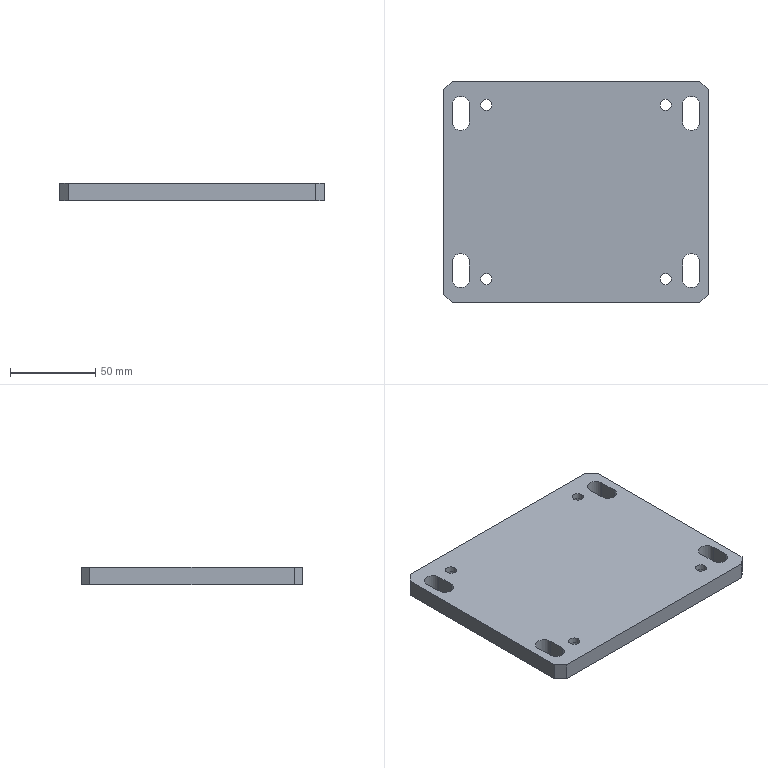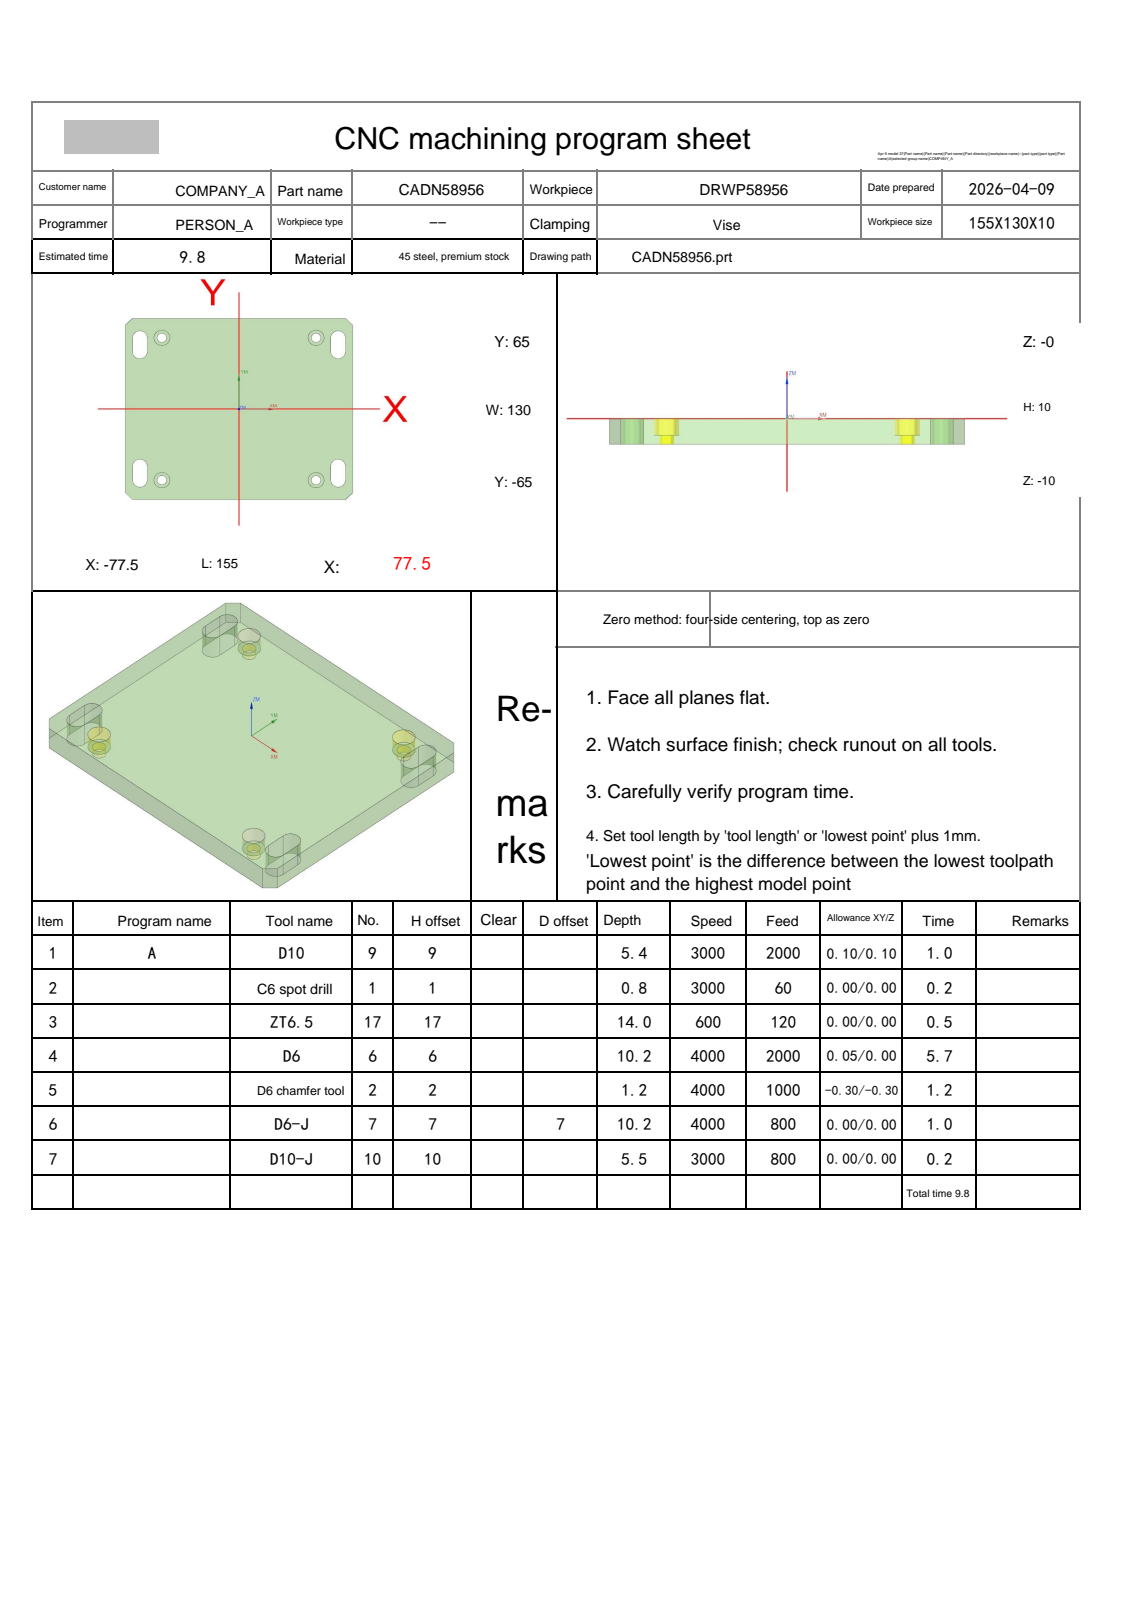NC program | NX | posted by the shop | part box 155 x 130 x 10 mm
Lines 1 to 1868 of 2515, first 1318 of 1866 lines:
%
O0001
(Machine time: 11.12 MIN)
(===Total Tool:7===)
(T9=D10     D=10.  R=0.   D-  H09 Z=-5.4  )
(T1=C6 spot drill   D=6.   R=0.   D-  H01 Z=-0.8  )
(T17=ZT6.5  D=6.5  DR_a=118 D-  H17 Z=-13.95)
(T6=D6      D=6.   R=0.   D-  H06 Z=-10.2 )
(T2=D6 chamfer tool   D=6.   R=0.   D-  H02 Z=-1.2  )
(T7=D6-J    D=6.   R=0.   D7  H07 Z=-10.2 )
(T10=D10-J  D=10.  R=0.   D-  H10 Z=-5.5  )
G80 G90 G17 G49 G40
G91 G28 Z0
M01
N1 T09 M06
(D10  D=10. R=0. H=09 ce=0.10 di=0.10)
G00 G90 G54 X-69.742 Y-74.97 M03 S3000
G43 H09 Z20.
M08
Z-.3
G01 X-76.106 Y-68.606 F2000.
X-81.106 Y-63.606
X-87.47 Y-57.242
G00 Z-.6
G01 X-81.106 Y-63.606
X-76.106 Y-68.606
X-69.742 Y-74.97
G00 Z-.9
G01 X-76.106 Y-68.606
X-81.106 Y-63.606
X-87.47 Y-57.242
G00 Z-1.2
G01 X-81.106 Y-63.606
X-76.106 Y-68.606
X-69.742 Y-74.97
G00 Z-1.5
G01 X-76.106 Y-68.606
X-81.106 Y-63.606
X-87.47 Y-57.242
G00 Z-1.8
G01 X-81.106 Y-63.606
X-76.106 Y-68.606
X-69.742 Y-74.97
G00 Z-2.1
G01 X-76.106 Y-68.606
X-81.106 Y-63.606
X-87.47 Y-57.242
G00 Z-2.4
G01 X-81.106 Y-63.606
X-76.106 Y-68.606
X-69.742 Y-74.97
G00 Z-2.7
G01 X-76.106 Y-68.606
X-81.106 Y-63.606
X-87.47 Y-57.242
G00 Z-3.
G01 X-81.106 Y-63.606
X-76.106 Y-68.606
X-69.742 Y-74.97
G00 Z-3.3
G01 X-76.106 Y-68.606
X-81.106 Y-63.606
X-87.47 Y-57.242
G00 Z-3.6
G01 X-81.106 Y-63.606
X-76.106 Y-68.606
X-69.742 Y-74.97
G00 Z-3.9
G01 X-76.106 Y-68.606
X-81.106 Y-63.606
X-87.47 Y-57.242
G00 Z-4.2
G01 X-81.106 Y-63.606
X-76.106 Y-68.606
X-69.742 Y-74.97
G00 Z-4.5
G01 X-76.106 Y-68.606
X-81.106 Y-63.606
X-87.47 Y-57.242
G00 Z-4.8
G01 X-81.106 Y-63.606
X-76.106 Y-68.606
X-69.742 Y-74.97
G00 Z-5.1
G01 X-76.106 Y-68.606
X-81.106 Y-63.606
X-87.47 Y-57.242
G00 Z-5.4
G01 X-81.106 Y-63.606
X-76.106 Y-68.606
X-69.742 Y-74.97
G00 Z20.
X-87.47 Y57.242
Z-.3
G01 X-81.106 Y63.606
X-76.106 Y68.606
X-69.742 Y74.97
G00 Z-.6
G01 X-76.106 Y68.606
X-81.106 Y63.606
X-87.47 Y57.242
G00 Z-.9
G01 X-81.106 Y63.606
X-76.106 Y68.606
X-69.742 Y74.97
G00 Z-1.2
G01 X-76.106 Y68.606
X-81.106 Y63.606
X-87.47 Y57.242
G00 Z-1.5
G01 X-81.106 Y63.606
X-76.106 Y68.606
X-69.742 Y74.97
G00 Z-1.8
G01 X-76.106 Y68.606
X-81.106 Y63.606
X-87.47 Y57.242
G00 Z-2.1
G01 X-81.106 Y63.606
X-76.106 Y68.606
X-69.742 Y74.97
G00 Z-2.4
G01 X-76.106 Y68.606
X-81.106 Y63.606
X-87.47 Y57.242
G00 Z-2.7
G01 X-81.106 Y63.606
X-76.106 Y68.606
X-69.742 Y74.97
G00 Z-3.
G01 X-76.106 Y68.606
X-81.106 Y63.606
X-87.47 Y57.242
G00 Z-3.3
G01 X-81.106 Y63.606
X-76.106 Y68.606
X-69.742 Y74.97
G00 Z-3.6
G01 X-76.106 Y68.606
X-81.106 Y63.606
X-87.47 Y57.242
G00 Z-3.9
G01 X-81.106 Y63.606
X-76.106 Y68.606
X-69.742 Y74.97
G00 Z-4.2
G01 X-76.106 Y68.606
X-81.106 Y63.606
X-87.47 Y57.242
G00 Z-4.5
G01 X-81.106 Y63.606
X-76.106 Y68.606
X-69.742 Y74.97
G00 Z-4.8
G01 X-76.106 Y68.606
X-81.106 Y63.606
X-87.47 Y57.242
G00 Z-5.1
G01 X-81.106 Y63.606
X-76.106 Y68.606
X-69.742 Y74.97
G00 Z-5.4
G01 X-76.106 Y68.606
X-81.106 Y63.606
X-87.47 Y57.242
G00 Z20.
X69.742 Y74.97
Z-.3
G01 X76.106 Y68.606
X81.106 Y63.606
X87.47 Y57.242
G00 Z-.6
G01 X81.106 Y63.606
X76.106 Y68.606
X69.742 Y74.97
G00 Z-.9
G01 X76.106 Y68.606
X81.106 Y63.606
X87.47 Y57.242
G00 Z-1.2
G01 X81.106 Y63.606
X76.106 Y68.606
X69.742 Y74.97
G00 Z-1.5
G01 X76.106 Y68.606
X81.106 Y63.606
X87.47 Y57.242
G00 Z-1.8
G01 X81.106 Y63.606
X76.106 Y68.606
X69.742 Y74.97
G00 Z-2.1
G01 X76.106 Y68.606
X81.106 Y63.606
X87.47 Y57.242
G00 Z-2.4
G01 X81.106 Y63.606
X76.106 Y68.606
X69.742 Y74.97
G00 Z-2.7
G01 X76.106 Y68.606
X81.106 Y63.606
X87.47 Y57.242
G00 Z-3.
G01 X81.106 Y63.606
X76.106 Y68.606
X69.742 Y74.97
G00 Z-3.3
G01 X76.106 Y68.606
X81.106 Y63.606
X87.47 Y57.242
G00 Z-3.6
G01 X81.106 Y63.606
X76.106 Y68.606
X69.742 Y74.97
G00 Z-3.9
G01 X76.106 Y68.606
X81.106 Y63.606
X87.47 Y57.242
G00 Z-4.2
G01 X81.106 Y63.606
X76.106 Y68.606
X69.742 Y74.97
G00 Z-4.5
G01 X76.106 Y68.606
X81.106 Y63.606
X87.47 Y57.242
G00 Z-4.8
G01 X81.106 Y63.606
X76.106 Y68.606
X69.742 Y74.97
G00 Z-5.1
G01 X76.106 Y68.606
X81.106 Y63.606
X87.47 Y57.242
G00 Z-5.4
G01 X81.106 Y63.606
X76.106 Y68.606
X69.742 Y74.97
G00 Z20.
X87.47 Y-57.242
Z-.3
G01 X81.106 Y-63.606
X76.106 Y-68.606
X69.742 Y-74.97
G00 Z-.6
G01 X76.106 Y-68.606
X81.106 Y-63.606
X87.47 Y-57.242
G00 Z-.9
G01 X81.106 Y-63.606
X76.106 Y-68.606
X69.742 Y-74.97
G00 Z-1.2
G01 X76.106 Y-68.606
X81.106 Y-63.606
X87.47 Y-57.242
G00 Z-1.5
G01 X81.106 Y-63.606
X76.106 Y-68.606
X69.742 Y-74.97
G00 Z-1.8
G01 X76.106 Y-68.606
X81.106 Y-63.606
X87.47 Y-57.242
G00 Z-2.1
G01 X81.106 Y-63.606
X76.106 Y-68.606
X69.742 Y-74.97
G00 Z-2.4
G01 X76.106 Y-68.606
X81.106 Y-63.606
X87.47 Y-57.242
G00 Z-2.7
G01 X81.106 Y-63.606
X76.106 Y-68.606
X69.742 Y-74.97
G00 Z-3.
G01 X76.106 Y-68.606
X81.106 Y-63.606
X87.47 Y-57.242
G00 Z-3.3
G01 X81.106 Y-63.606
X76.106 Y-68.606
X69.742 Y-74.97
G00 Z-3.6
G01 X76.106 Y-68.606
X81.106 Y-63.606
X87.47 Y-57.242
G00 Z-3.9
G01 X81.106 Y-63.606
X76.106 Y-68.606
X69.742 Y-74.97
G00 Z-4.2
G01 X76.106 Y-68.606
X81.106 Y-63.606
X87.47 Y-57.242
G00 Z-4.5
G01 X81.106 Y-63.606
X76.106 Y-68.606
X69.742 Y-74.97
G00 Z-4.8
G01 X76.106 Y-68.606
X81.106 Y-63.606
X87.47 Y-57.242
G00 Z-5.1
G01 X81.106 Y-63.606
X76.106 Y-68.606
X69.742 Y-74.97
G00 Z-5.4
G01 X76.106 Y-68.606
X81.106 Y-63.606
X87.47 Y-57.242
G00 Z20.
G91 G28 Z0.0
M05
M09
G91 G28 Z0.0
M01
N2 T01 M06
(C6 spot drill D=6. R=0. H=01 ce=0.00 di=0.10)
G00 G90 G54 X-52.5 Y-51. M03 S3000
G43 H01 Z20.
M08
G98 G81 X-52.5 Y-51. Z-.8 R1. F60.
Y51.
X52.5
Y-51.
G80
G00 Z20.
G91 G28 Z0.0
M05
M09
G91 G28 Z0.0
M01
N3 T17 M06
(ZT6.5 D=6.5 DR_a=118 H=17)
G00 G90 G54 X-52.5 Y-51. M03 S600
G43 H17 Z20.
M08
G98 G83 X-52.5 Y-51. Z-13.953 R1. F120. Q2.
Y51.
X52.5
Y-51.
G80
G00 Z20.
G91 G28 Z0.0
M05
M09
G91 G28 Z0.0
M01
N4 T06 M06
(D6  D=6. R=0. H=06 ce=0.05 di=0.10)
G00 G90 G54 X-67.311 Y-52.95 M03 S4000
G43 H06 Z20.
M08
Z1.
G01 X-67.157 Z.992 F1500.
X-66.412 Y-52.654 Z.95
X-65.846 Y-52.088 Z.908
X-65.55 Y-51.343 Z.866
Y-40.657 Z.306
X-65.846 Y-39.912 Z.264
X-66.412 Y-39.346 Z.222
X-67.157 Y-39.05 Z.18
X-67.843 Z.144
X-68.588 Y-39.346 Z.102
X-69.154 Y-39.912 Z.06
X-69.45 Y-40.657 Z.018
Y-41. Z0.0
Y-51. Z-.062
G03 X-67.5 Y-52.95 Z-.081 I1.95 J0.0
X-65.55 Y-51. Z-.1 I0.0 J1.95
G01 Y-41. Z-.162
G03 X-67.5 Y-39.05 Z-.181 I-1.95 J0.0
X-69.45 Y-41. Z-.2 I0.0 J-1.95
G01 Y-51. Z-.262
G03 X-67.5 Y-52.95 Z-.281 I1.95 J0.0
X-65.55 Y-51. Z-.3 I0.0 J1.95
G01 Y-41. Z-.362
G03 X-67.5 Y-39.05 Z-.381 I-1.95 J0.0
X-69.45 Y-41. Z-.4 I0.0 J-1.95
G01 Y-51. Z-.462
G03 X-67.5 Y-52.95 Z-.481 I1.95 J0.0
X-65.55 Y-51. Z-.5 I0.0 J1.95
G01 Y-41. Z-.562
G03 X-67.5 Y-39.05 Z-.581 I-1.95 J0.0
X-69.45 Y-41. Z-.6 I0.0 J-1.95
G01 Y-51. Z-.662
G03 X-67.5 Y-52.95 Z-.681 I1.95 J0.0
X-65.55 Y-51. Z-.7 I0.0 J1.95
G01 Y-41. Z-.762
G03 X-67.5 Y-39.05 Z-.781 I-1.95 J0.0
X-69.45 Y-41. Z-.8 I0.0 J-1.95
G01 Y-51. Z-.862
G03 X-67.5 Y-52.95 Z-.881 I1.95 J0.0
X-65.55 Y-51. Z-.9 I0.0 J1.95
G01 Y-41. Z-.962
G03 X-67.5 Y-39.05 Z-.981 I-1.95 J0.0
X-69.45 Y-41. Z-1. I0.0 J-1.95
G01 Y-51. Z-1.062
G03 X-67.5 Y-52.95 Z-1.081 I1.95 J0.0
X-65.55 Y-51. Z-1.1 I0.0 J1.95
G01 Y-41. Z-1.162
G03 X-67.5 Y-39.05 Z-1.181 I-1.95 J0.0
X-69.45 Y-41. Z-1.2 I0.0 J-1.95
G01 Y-51. Z-1.262
G03 X-67.5 Y-52.95 Z-1.281 I1.95 J0.0
X-65.55 Y-51. Z-1.3 I0.0 J1.95
G01 Y-41. Z-1.362
G03 X-67.5 Y-39.05 Z-1.381 I-1.95 J0.0
X-69.45 Y-41. Z-1.4 I0.0 J-1.95
G01 Y-51. Z-1.462
G03 X-67.5 Y-52.95 Z-1.481 I1.95 J0.0
X-65.55 Y-51. Z-1.5 I0.0 J1.95
G01 Y-41. Z-1.562
G03 X-67.5 Y-39.05 Z-1.581 I-1.95 J0.0
X-69.45 Y-41. Z-1.6 I0.0 J-1.95
G01 Y-51. Z-1.662
G03 X-67.5 Y-52.95 Z-1.681 I1.95 J0.0
X-65.55 Y-51. Z-1.7 I0.0 J1.95
G01 Y-41. Z-1.762
G03 X-67.5 Y-39.05 Z-1.781 I-1.95 J0.0
X-69.45 Y-41. Z-1.8 I0.0 J-1.95
G01 Y-51. Z-1.862
G03 X-67.5 Y-52.95 Z-1.881 I1.95 J0.0
X-65.55 Y-51. Z-1.9 I0.0 J1.95
G01 Y-41. Z-1.962
G03 X-67.5 Y-39.05 Z-1.981 I-1.95 J0.0
X-69.45 Y-41. Z-2. I0.0 J-1.95
G01 Y-51. Z-2.062
G03 X-67.5 Y-52.95 Z-2.081 I1.95 J0.0
X-65.55 Y-51. Z-2.1 I0.0 J1.95
G01 Y-41. Z-2.162
G03 X-67.5 Y-39.05 Z-2.181 I-1.95 J0.0
X-69.45 Y-41. Z-2.2 I0.0 J-1.95
G01 Y-51. Z-2.262
G03 X-67.5 Y-52.95 Z-2.281 I1.95 J0.0
X-65.55 Y-51. Z-2.3 I0.0 J1.95
G01 Y-41. Z-2.362
G03 X-67.5 Y-39.05 Z-2.381 I-1.95 J0.0
X-69.45 Y-41. Z-2.4 I0.0 J-1.95
G01 Y-51. Z-2.462
G03 X-67.5 Y-52.95 Z-2.481 I1.95 J0.0
X-65.55 Y-51. Z-2.5 I0.0 J1.95
G01 Y-41. Z-2.562
G03 X-67.5 Y-39.05 Z-2.581 I-1.95 J0.0
X-69.45 Y-41. Z-2.6 I0.0 J-1.95
G01 Y-51. Z-2.662
G03 X-67.5 Y-52.95 Z-2.681 I1.95 J0.0
X-65.55 Y-51. Z-2.7 I0.0 J1.95
G01 Y-41. Z-2.762
G03 X-67.5 Y-39.05 Z-2.781 I-1.95 J0.0
X-69.45 Y-41. Z-2.8 I0.0 J-1.95
G01 Y-51. Z-2.862
G03 X-67.5 Y-52.95 Z-2.881 I1.95 J0.0
X-65.55 Y-51. Z-2.9 I0.0 J1.95
G01 Y-41. Z-2.962
G03 X-67.5 Y-39.05 Z-2.981 I-1.95 J0.0
X-69.45 Y-41. Z-3. I0.0 J-1.95
G01 Y-51. Z-3.062
G03 X-67.5 Y-52.95 Z-3.081 I1.95 J0.0
X-65.55 Y-51. Z-3.1 I0.0 J1.95
G01 Y-41. Z-3.162
G03 X-67.5 Y-39.05 Z-3.181 I-1.95 J0.0
X-69.45 Y-41. Z-3.2 I0.0 J-1.95
G01 Y-51. Z-3.262
G03 X-67.5 Y-52.95 Z-3.281 I1.95 J0.0
X-65.55 Y-51. Z-3.3 I0.0 J1.95
G01 Y-41. Z-3.362
G03 X-67.5 Y-39.05 Z-3.381 I-1.95 J0.0
X-69.45 Y-41. Z-3.4 I0.0 J-1.95
G01 Y-51. Z-3.462
G03 X-67.5 Y-52.95 Z-3.481 I1.95 J0.0
X-65.55 Y-51. Z-3.5 I0.0 J1.95
G01 Y-41. Z-3.562
G03 X-67.5 Y-39.05 Z-3.581 I-1.95 J0.0
X-69.45 Y-41. Z-3.6 I0.0 J-1.95
G01 Y-51. Z-3.662
G03 X-67.5 Y-52.95 Z-3.681 I1.95 J0.0
X-65.55 Y-51. Z-3.7 I0.0 J1.95
G01 Y-41. Z-3.762
G03 X-67.5 Y-39.05 Z-3.781 I-1.95 J0.0
X-69.45 Y-41. Z-3.8 I0.0 J-1.95
G01 Y-51. Z-3.862
G03 X-67.5 Y-52.95 Z-3.881 I1.95 J0.0
X-65.55 Y-51. Z-3.9 I0.0 J1.95
G01 Y-41. Z-3.962
G03 X-67.5 Y-39.05 Z-3.981 I-1.95 J0.0
X-69.45 Y-41. Z-4. I0.0 J-1.95
G01 Y-51. Z-4.062
G03 X-67.5 Y-52.95 Z-4.081 I1.95 J0.0
X-65.55 Y-51. Z-4.1 I0.0 J1.95
G01 Y-41. Z-4.162
G03 X-67.5 Y-39.05 Z-4.181 I-1.95 J0.0
X-69.45 Y-41. Z-4.2 I0.0 J-1.95
G01 Y-51. Z-4.262
G03 X-67.5 Y-52.95 Z-4.281 I1.95 J0.0
X-65.55 Y-51. Z-4.3 I0.0 J1.95
G01 Y-41. Z-4.362
G03 X-67.5 Y-39.05 Z-4.381 I-1.95 J0.0
X-69.45 Y-41. Z-4.4 I0.0 J-1.95
G01 Y-51. Z-4.462
G03 X-67.5 Y-52.95 Z-4.481 I1.95 J0.0
X-65.55 Y-51. Z-4.5 I0.0 J1.95
G01 Y-41. Z-4.562
G03 X-67.5 Y-39.05 Z-4.581 I-1.95 J0.0
X-69.45 Y-41. Z-4.6 I0.0 J-1.95
G01 Y-51. Z-4.662
G03 X-67.5 Y-52.95 Z-4.681 I1.95 J0.0
X-65.55 Y-51. Z-4.7 I0.0 J1.95
G01 Y-41. Z-4.762
G03 X-67.5 Y-39.05 Z-4.781 I-1.95 J0.0
X-69.45 Y-41. Z-4.8 I0.0 J-1.95
G01 Y-51. Z-4.862
G03 X-67.5 Y-52.95 Z-4.881 I1.95 J0.0
X-65.55 Y-51. Z-4.9 I0.0 J1.95
G01 Y-41. Z-4.962
G03 X-67.5 Y-39.05 Z-4.981 I-1.95 J0.0
X-69.45 Y-41. Z-5. I0.0 J-1.95
G01 Y-51. Z-5.062
G03 X-67.5 Y-52.95 Z-5.081 I1.95 J0.0
X-65.55 Y-51. Z-5.1 I0.0 J1.95
G01 Y-41. Z-5.162
G03 X-67.5 Y-39.05 Z-5.181 I-1.95 J0.0
X-69.45 Y-41. Z-5.2 I0.0 J-1.95
G01 Y-51. Z-5.262
G03 X-67.5 Y-52.95 Z-5.281 I1.95 J0.0
X-65.55 Y-51. Z-5.3 I0.0 J1.95
G01 Y-41. Z-5.362
G03 X-67.5 Y-39.05 Z-5.381 I-1.95 J0.0
X-69.45 Y-41. Z-5.4 I0.0 J-1.95
G01 Y-51. Z-5.462
G03 X-67.5 Y-52.95 Z-5.481 I1.95 J0.0
X-65.55 Y-51. Z-5.5 I0.0 J1.95
G01 Y-41. Z-5.562
G03 X-67.5 Y-39.05 Z-5.581 I-1.95 J0.0
X-69.45 Y-41. Z-5.6 I0.0 J-1.95
G01 Y-51. Z-5.662
G03 X-67.5 Y-52.95 Z-5.681 I1.95 J0.0
X-65.55 Y-51. Z-5.7 I0.0 J1.95
G01 Y-41. Z-5.762
G03 X-67.5 Y-39.05 Z-5.781 I-1.95 J0.0
X-69.45 Y-41. Z-5.8 I0.0 J-1.95
G01 Y-51. Z-5.862
G03 X-67.5 Y-52.95 Z-5.881 I1.95 J0.0
X-65.55 Y-51. Z-5.9 I0.0 J1.95
G01 Y-41. Z-5.962
G03 X-67.5 Y-39.05 Z-5.981 I-1.95 J0.0
X-69.45 Y-41. Z-6. I0.0 J-1.95
G01 Y-51. Z-6.062
G03 X-67.5 Y-52.95 Z-6.081 I1.95 J0.0
X-65.55 Y-51. Z-6.1 I0.0 J1.95
G01 Y-41. Z-6.162
G03 X-67.5 Y-39.05 Z-6.181 I-1.95 J0.0
X-69.45 Y-41. Z-6.2 I0.0 J-1.95
G01 Y-51. Z-6.262
G03 X-67.5 Y-52.95 Z-6.281 I1.95 J0.0
X-65.55 Y-51. Z-6.3 I0.0 J1.95
G01 Y-41. Z-6.362
G03 X-67.5 Y-39.05 Z-6.381 I-1.95 J0.0
X-69.45 Y-41. Z-6.4 I0.0 J-1.95
G01 Y-51. Z-6.462
G03 X-67.5 Y-52.95 Z-6.481 I1.95 J0.0
X-65.55 Y-51. Z-6.5 I0.0 J1.95
G01 Y-41. Z-6.562
G03 X-67.5 Y-39.05 Z-6.581 I-1.95 J0.0
X-69.45 Y-41. Z-6.6 I0.0 J-1.95
G01 Y-51. Z-6.662
G03 X-67.5 Y-52.95 Z-6.681 I1.95 J0.0
X-65.55 Y-51. Z-6.7 I0.0 J1.95
G01 Y-41. Z-6.762
G03 X-67.5 Y-39.05 Z-6.781 I-1.95 J0.0
X-69.45 Y-41. Z-6.8 I0.0 J-1.95
G01 Y-51. Z-6.862
G03 X-67.5 Y-52.95 Z-6.881 I1.95 J0.0
X-65.55 Y-51. Z-6.9 I0.0 J1.95
G01 Y-41. Z-6.962
G03 X-67.5 Y-39.05 Z-6.981 I-1.95 J0.0
X-69.45 Y-41. Z-7. I0.0 J-1.95
G01 Y-51. Z-7.062
G03 X-67.5 Y-52.95 Z-7.081 I1.95 J0.0
X-65.55 Y-51. Z-7.1 I0.0 J1.95
G01 Y-41. Z-7.162
G03 X-67.5 Y-39.05 Z-7.181 I-1.95 J0.0
X-69.45 Y-41. Z-7.2 I0.0 J-1.95
G01 Y-51. Z-7.262
G03 X-67.5 Y-52.95 Z-7.281 I1.95 J0.0
X-65.55 Y-51. Z-7.3 I0.0 J1.95
G01 Y-41. Z-7.362
G03 X-67.5 Y-39.05 Z-7.381 I-1.95 J0.0
X-69.45 Y-41. Z-7.4 I0.0 J-1.95
G01 Y-51. Z-7.462
G03 X-67.5 Y-52.95 Z-7.481 I1.95 J0.0
X-65.55 Y-51. Z-7.5 I0.0 J1.95
G01 Y-41. Z-7.562
G03 X-67.5 Y-39.05 Z-7.581 I-1.95 J0.0
X-69.45 Y-41. Z-7.6 I0.0 J-1.95
G01 Y-51. Z-7.662
G03 X-67.5 Y-52.95 Z-7.681 I1.95 J0.0
X-65.55 Y-51. Z-7.7 I0.0 J1.95
G01 Y-41. Z-7.762
G03 X-67.5 Y-39.05 Z-7.781 I-1.95 J0.0
X-69.45 Y-41. Z-7.8 I0.0 J-1.95
G01 Y-51. Z-7.862
G03 X-67.5 Y-52.95 Z-7.881 I1.95 J0.0
X-65.55 Y-51. Z-7.9 I0.0 J1.95
G01 Y-41. Z-7.962
G03 X-67.5 Y-39.05 Z-7.981 I-1.95 J0.0
X-69.45 Y-41. Z-8. I0.0 J-1.95
G01 Y-51. Z-8.062
G03 X-67.5 Y-52.95 Z-8.081 I1.95 J0.0
X-65.55 Y-51. Z-8.1 I0.0 J1.95
G01 Y-41. Z-8.162
G03 X-67.5 Y-39.05 Z-8.181 I-1.95 J0.0
X-69.45 Y-41. Z-8.2 I0.0 J-1.95
G01 Y-51. Z-8.262
G03 X-67.5 Y-52.95 Z-8.281 I1.95 J0.0
X-65.55 Y-51. Z-8.3 I0.0 J1.95
G01 Y-41. Z-8.362
G03 X-67.5 Y-39.05 Z-8.381 I-1.95 J0.0
X-69.45 Y-41. Z-8.4 I0.0 J-1.95
G01 Y-51. Z-8.462
G03 X-67.5 Y-52.95 Z-8.481 I1.95 J0.0
X-65.55 Y-51. Z-8.5 I0.0 J1.95
G01 Y-41. Z-8.562
G03 X-67.5 Y-39.05 Z-8.581 I-1.95 J0.0
X-69.45 Y-41. Z-8.6 I0.0 J-1.95
G01 Y-51. Z-8.662
G03 X-67.5 Y-52.95 Z-8.681 I1.95 J0.0
X-65.55 Y-51. Z-8.7 I0.0 J1.95
G01 Y-41. Z-8.762
G03 X-67.5 Y-39.05 Z-8.781 I-1.95 J0.0
X-69.45 Y-41. Z-8.8 I0.0 J-1.95
G01 Y-51. Z-8.862
G03 X-67.5 Y-52.95 Z-8.881 I1.95 J0.0
X-65.55 Y-51. Z-8.9 I0.0 J1.95
G01 Y-41. Z-8.962
G03 X-67.5 Y-39.05 Z-8.981 I-1.95 J0.0
X-69.45 Y-41. Z-9. I0.0 J-1.95
G01 Y-51. Z-9.062
G03 X-67.5 Y-52.95 Z-9.081 I1.95 J0.0
X-65.55 Y-51. Z-9.1 I0.0 J1.95
G01 Y-41. Z-9.162
G03 X-67.5 Y-39.05 Z-9.181 I-1.95 J0.0
X-69.45 Y-41. Z-9.2 I0.0 J-1.95
G01 Y-51. Z-9.262
G03 X-67.5 Y-52.95 Z-9.281 I1.95 J0.0
X-65.55 Y-51. Z-9.3 I0.0 J1.95
G01 Y-41. Z-9.362
G03 X-67.5 Y-39.05 Z-9.381 I-1.95 J0.0
X-69.45 Y-41. Z-9.4 I0.0 J-1.95
G01 Y-51. Z-9.462
G03 X-67.5 Y-52.95 Z-9.481 I1.95 J0.0
X-65.55 Y-51. Z-9.5 I0.0 J1.95
G01 Y-41. Z-9.562
G03 X-67.5 Y-39.05 Z-9.581 I-1.95 J0.0
X-69.45 Y-41. Z-9.6 I0.0 J-1.95
G01 Y-51. Z-9.662
G03 X-67.5 Y-52.95 Z-9.681 I1.95 J0.0
X-65.55 Y-51. Z-9.7 I0.0 J1.95
G01 Y-41. Z-9.762
G03 X-67.5 Y-39.05 Z-9.781 I-1.95 J0.0
X-69.45 Y-41. Z-9.8 I0.0 J-1.95
G01 Y-51. Z-9.862
G03 X-67.5 Y-52.95 Z-9.881 I1.95 J0.0
X-65.55 Y-51. Z-9.9 I0.0 J1.95
G01 Y-41. Z-9.962
G03 X-67.5 Y-39.05 Z-9.981 I-1.95 J0.0
X-69.45 Y-41. Z-10. I0.0 J-1.95
G01 Y-51. Z-10.062
G03 X-67.5 Y-52.95 Z-10.081 I1.95 J0.0
X-65.55 Y-51. Z-10.1 I0.0 J1.95
G01 Y-41. Z-10.162
G03 X-67.5 Y-39.05 Z-10.181 I-1.95 J0.0
X-69.45 Y-41. Z-10.2 I0.0 J-1.95
G01 Y-51.
G03 X-67.5 Y-52.95 I1.95 J0.0
X-65.55 Y-51. I0.0 J1.95
G01 Y-41.
G03 X-67.5 Y-39.05 I-1.95 J0.0
X-69.45 Y-41. I0.0 J-1.95
G01 Y-41.4
Z-9.2
G00 Z20.
X-67.311 Y39.05
Z1.
G01 X-67.157 Z.992
X-66.412 Y39.346 Z.95
X-65.846 Y39.912 Z.908
X-65.55 Y40.657 Z.866
Y51.343 Z.306
X-65.846 Y52.088 Z.264
X-66.412 Y52.654 Z.222
X-67.157 Y52.95 Z.18
X-67.843 Z.144
X-68.588 Y52.654 Z.102
X-69.154 Y52.088 Z.06
X-69.45 Y51.343 Z.018
Y51. Z0.0
Y41. Z-.062
G03 X-67.5 Y39.05 Z-.081 I1.95 J0.0
X-65.55 Y41. Z-.1 I0.0 J1.95
G01 Y51. Z-.162
G03 X-67.5 Y52.95 Z-.181 I-1.95 J0.0
X-69.45 Y51. Z-.2 I0.0 J-1.95
G01 Y41. Z-.262
G03 X-67.5 Y39.05 Z-.281 I1.95 J0.0
X-65.55 Y41. Z-.3 I0.0 J1.95
G01 Y51. Z-.362
G03 X-67.5 Y52.95 Z-.381 I-1.95 J0.0
X-69.45 Y51. Z-.4 I0.0 J-1.95
G01 Y41. Z-.462
G03 X-67.5 Y39.05 Z-.481 I1.95 J0.0
X-65.55 Y41. Z-.5 I0.0 J1.95
G01 Y51. Z-.562
G03 X-67.5 Y52.95 Z-.581 I-1.95 J0.0
X-69.45 Y51. Z-.6 I0.0 J-1.95
G01 Y41. Z-.662
G03 X-67.5 Y39.05 Z-.681 I1.95 J0.0
X-65.55 Y41. Z-.7 I0.0 J1.95
G01 Y51. Z-.762
G03 X-67.5 Y52.95 Z-.781 I-1.95 J0.0
X-69.45 Y51. Z-.8 I0.0 J-1.95
G01 Y41. Z-.862
G03 X-67.5 Y39.05 Z-.881 I1.95 J0.0
X-65.55 Y41. Z-.9 I0.0 J1.95
G01 Y51. Z-.962
G03 X-67.5 Y52.95 Z-.981 I-1.95 J0.0
X-69.45 Y51. Z-1. I0.0 J-1.95
G01 Y41. Z-1.062
G03 X-67.5 Y39.05 Z-1.081 I1.95 J0.0
X-65.55 Y41. Z-1.1 I0.0 J1.95
G01 Y51. Z-1.162
G03 X-67.5 Y52.95 Z-1.181 I-1.95 J0.0
X-69.45 Y51. Z-1.2 I0.0 J-1.95
G01 Y41. Z-1.262
G03 X-67.5 Y39.05 Z-1.281 I1.95 J0.0
X-65.55 Y41. Z-1.3 I0.0 J1.95
G01 Y51. Z-1.362
G03 X-67.5 Y52.95 Z-1.381 I-1.95 J0.0
X-69.45 Y51. Z-1.4 I0.0 J-1.95
G01 Y41. Z-1.462
G03 X-67.5 Y39.05 Z-1.481 I1.95 J0.0
X-65.55 Y41. Z-1.5 I0.0 J1.95
G01 Y51. Z-1.562
G03 X-67.5 Y52.95 Z-1.581 I-1.95 J0.0
X-69.45 Y51. Z-1.6 I0.0 J-1.95
G01 Y41. Z-1.662
G03 X-67.5 Y39.05 Z-1.681 I1.95 J0.0
X-65.55 Y41. Z-1.7 I0.0 J1.95
G01 Y51. Z-1.762
G03 X-67.5 Y52.95 Z-1.781 I-1.95 J0.0
X-69.45 Y51. Z-1.8 I0.0 J-1.95
G01 Y41. Z-1.862
G03 X-67.5 Y39.05 Z-1.881 I1.95 J0.0
X-65.55 Y41. Z-1.9 I0.0 J1.95
G01 Y51. Z-1.962
G03 X-67.5 Y52.95 Z-1.981 I-1.95 J0.0
X-69.45 Y51. Z-2. I0.0 J-1.95
G01 Y41. Z-2.062
G03 X-67.5 Y39.05 Z-2.081 I1.95 J0.0
X-65.55 Y41. Z-2.1 I0.0 J1.95
G01 Y51. Z-2.162
G03 X-67.5 Y52.95 Z-2.181 I-1.95 J0.0
X-69.45 Y51. Z-2.2 I0.0 J-1.95
G01 Y41. Z-2.262
G03 X-67.5 Y39.05 Z-2.281 I1.95 J0.0
X-65.55 Y41. Z-2.3 I0.0 J1.95
G01 Y51. Z-2.362
G03 X-67.5 Y52.95 Z-2.381 I-1.95 J0.0
X-69.45 Y51. Z-2.4 I0.0 J-1.95
G01 Y41. Z-2.462
G03 X-67.5 Y39.05 Z-2.481 I1.95 J0.0
X-65.55 Y41. Z-2.5 I0.0 J1.95
G01 Y51. Z-2.562
G03 X-67.5 Y52.95 Z-2.581 I-1.95 J0.0
X-69.45 Y51. Z-2.6 I0.0 J-1.95
G01 Y41. Z-2.662
G03 X-67.5 Y39.05 Z-2.681 I1.95 J0.0
X-65.55 Y41. Z-2.7 I0.0 J1.95
G01 Y51. Z-2.762
G03 X-67.5 Y52.95 Z-2.781 I-1.95 J0.0
X-69.45 Y51. Z-2.8 I0.0 J-1.95
G01 Y41. Z-2.862
G03 X-67.5 Y39.05 Z-2.881 I1.95 J0.0
X-65.55 Y41. Z-2.9 I0.0 J1.95
G01 Y51. Z-2.962
G03 X-67.5 Y52.95 Z-2.981 I-1.95 J0.0
X-69.45 Y51. Z-3. I0.0 J-1.95
G01 Y41. Z-3.062
G03 X-67.5 Y39.05 Z-3.081 I1.95 J0.0
X-65.55 Y41. Z-3.1 I0.0 J1.95
G01 Y51. Z-3.162
G03 X-67.5 Y52.95 Z-3.181 I-1.95 J0.0
X-69.45 Y51. Z-3.2 I0.0 J-1.95
G01 Y41. Z-3.262
G03 X-67.5 Y39.05 Z-3.281 I1.95 J0.0
X-65.55 Y41. Z-3.3 I0.0 J1.95
G01 Y51. Z-3.362
G03 X-67.5 Y52.95 Z-3.381 I-1.95 J0.0
X-69.45 Y51. Z-3.4 I0.0 J-1.95
G01 Y41. Z-3.462
G03 X-67.5 Y39.05 Z-3.481 I1.95 J0.0
X-65.55 Y41. Z-3.5 I0.0 J1.95
G01 Y51. Z-3.562
G03 X-67.5 Y52.95 Z-3.581 I-1.95 J0.0
X-69.45 Y51. Z-3.6 I0.0 J-1.95
G01 Y41. Z-3.662
G03 X-67.5 Y39.05 Z-3.681 I1.95 J0.0
X-65.55 Y41. Z-3.7 I0.0 J1.95
G01 Y51. Z-3.762
G03 X-67.5 Y52.95 Z-3.781 I-1.95 J0.0
X-69.45 Y51. Z-3.8 I0.0 J-1.95
G01 Y41. Z-3.862
G03 X-67.5 Y39.05 Z-3.881 I1.95 J0.0
X-65.55 Y41. Z-3.9 I0.0 J1.95
G01 Y51. Z-3.962
G03 X-67.5 Y52.95 Z-3.981 I-1.95 J0.0
X-69.45 Y51. Z-4. I0.0 J-1.95
G01 Y41. Z-4.062
G03 X-67.5 Y39.05 Z-4.081 I1.95 J0.0
X-65.55 Y41. Z-4.1 I0.0 J1.95
G01 Y51. Z-4.162
G03 X-67.5 Y52.95 Z-4.181 I-1.95 J0.0
X-69.45 Y51. Z-4.2 I0.0 J-1.95
G01 Y41. Z-4.262
G03 X-67.5 Y39.05 Z-4.281 I1.95 J0.0
X-65.55 Y41. Z-4.3 I0.0 J1.95
G01 Y51. Z-4.362
G03 X-67.5 Y52.95 Z-4.381 I-1.95 J0.0
X-69.45 Y51. Z-4.4 I0.0 J-1.95
G01 Y41. Z-4.462
G03 X-67.5 Y39.05 Z-4.481 I1.95 J0.0
X-65.55 Y41. Z-4.5 I0.0 J1.95
G01 Y51. Z-4.562
G03 X-67.5 Y52.95 Z-4.581 I-1.95 J0.0
X-69.45 Y51. Z-4.6 I0.0 J-1.95
G01 Y41. Z-4.662
G03 X-67.5 Y39.05 Z-4.681 I1.95 J0.0
X-65.55 Y41. Z-4.7 I0.0 J1.95
G01 Y51. Z-4.762
G03 X-67.5 Y52.95 Z-4.781 I-1.95 J0.0
X-69.45 Y51. Z-4.8 I0.0 J-1.95
G01 Y41. Z-4.862
G03 X-67.5 Y39.05 Z-4.881 I1.95 J0.0
X-65.55 Y41. Z-4.9 I0.0 J1.95
G01 Y51. Z-4.962
G03 X-67.5 Y52.95 Z-4.981 I-1.95 J0.0
X-69.45 Y51. Z-5. I0.0 J-1.95
G01 Y41. Z-5.062
G03 X-67.5 Y39.05 Z-5.081 I1.95 J0.0
X-65.55 Y41. Z-5.1 I0.0 J1.95
G01 Y51. Z-5.162
G03 X-67.5 Y52.95 Z-5.181 I-1.95 J0.0
X-69.45 Y51. Z-5.2 I0.0 J-1.95
G01 Y41. Z-5.262
G03 X-67.5 Y39.05 Z-5.281 I1.95 J0.0
X-65.55 Y41. Z-5.3 I0.0 J1.95
G01 Y51. Z-5.362
G03 X-67.5 Y52.95 Z-5.381 I-1.95 J0.0
X-69.45 Y51. Z-5.4 I0.0 J-1.95
G01 Y41. Z-5.462
G03 X-67.5 Y39.05 Z-5.481 I1.95 J0.0
X-65.55 Y41. Z-5.5 I0.0 J1.95
G01 Y51. Z-5.562
G03 X-67.5 Y52.95 Z-5.581 I-1.95 J0.0
X-69.45 Y51. Z-5.6 I0.0 J-1.95
G01 Y41. Z-5.662
G03 X-67.5 Y39.05 Z-5.681 I1.95 J0.0
X-65.55 Y41. Z-5.7 I0.0 J1.95
G01 Y51. Z-5.762
G03 X-67.5 Y52.95 Z-5.781 I-1.95 J0.0
X-69.45 Y51. Z-5.8 I0.0 J-1.95
G01 Y41. Z-5.862
G03 X-67.5 Y39.05 Z-5.881 I1.95 J0.0
X-65.55 Y41. Z-5.9 I0.0 J1.95
G01 Y51. Z-5.962
G03 X-67.5 Y52.95 Z-5.981 I-1.95 J0.0
X-69.45 Y51. Z-6. I0.0 J-1.95
G01 Y41. Z-6.062
G03 X-67.5 Y39.05 Z-6.081 I1.95 J0.0
X-65.55 Y41. Z-6.1 I0.0 J1.95
G01 Y51. Z-6.162
G03 X-67.5 Y52.95 Z-6.181 I-1.95 J0.0
X-69.45 Y51. Z-6.2 I0.0 J-1.95
G01 Y41. Z-6.262
G03 X-67.5 Y39.05 Z-6.281 I1.95 J0.0
X-65.55 Y41. Z-6.3 I0.0 J1.95
G01 Y51. Z-6.362
G03 X-67.5 Y52.95 Z-6.381 I-1.95 J0.0
X-69.45 Y51. Z-6.4 I0.0 J-1.95
G01 Y41. Z-6.462
G03 X-67.5 Y39.05 Z-6.481 I1.95 J0.0
X-65.55 Y41. Z-6.5 I0.0 J1.95
G01 Y51. Z-6.562
G03 X-67.5 Y52.95 Z-6.581 I-1.95 J0.0
X-69.45 Y51. Z-6.6 I0.0 J-1.95
G01 Y41. Z-6.662
G03 X-67.5 Y39.05 Z-6.681 I1.95 J0.0
X-65.55 Y41. Z-6.7 I0.0 J1.95
G01 Y51. Z-6.762
G03 X-67.5 Y52.95 Z-6.781 I-1.95 J0.0
X-69.45 Y51. Z-6.8 I0.0 J-1.95
G01 Y41. Z-6.862
G03 X-67.5 Y39.05 Z-6.881 I1.95 J0.0
X-65.55 Y41. Z-6.9 I0.0 J1.95
G01 Y51. Z-6.962
G03 X-67.5 Y52.95 Z-6.981 I-1.95 J0.0
X-69.45 Y51. Z-7. I0.0 J-1.95
G01 Y41. Z-7.062
G03 X-67.5 Y39.05 Z-7.081 I1.95 J0.0
X-65.55 Y41. Z-7.1 I0.0 J1.95
G01 Y51. Z-7.162
G03 X-67.5 Y52.95 Z-7.181 I-1.95 J0.0
X-69.45 Y51. Z-7.2 I0.0 J-1.95
G01 Y41. Z-7.262
G03 X-67.5 Y39.05 Z-7.281 I1.95 J0.0
X-65.55 Y41. Z-7.3 I0.0 J1.95
G01 Y51. Z-7.362
G03 X-67.5 Y52.95 Z-7.381 I-1.95 J0.0
X-69.45 Y51. Z-7.4 I0.0 J-1.95
G01 Y41. Z-7.462
G03 X-67.5 Y39.05 Z-7.481 I1.95 J0.0
X-65.55 Y41. Z-7.5 I0.0 J1.95
G01 Y51. Z-7.562
G03 X-67.5 Y52.95 Z-7.581 I-1.95 J0.0
X-69.45 Y51. Z-7.6 I0.0 J-1.95
G01 Y41. Z-7.662
G03 X-67.5 Y39.05 Z-7.681 I1.95 J0.0
X-65.55 Y41. Z-7.7 I0.0 J1.95
G01 Y51. Z-7.762
G03 X-67.5 Y52.95 Z-7.781 I-1.95 J0.0
X-69.45 Y51. Z-7.8 I0.0 J-1.95
G01 Y41. Z-7.862
G03 X-67.5 Y39.05 Z-7.881 I1.95 J0.0
X-65.55 Y41. Z-7.9 I0.0 J1.95
G01 Y51. Z-7.962
G03 X-67.5 Y52.95 Z-7.981 I-1.95 J0.0
X-69.45 Y51. Z-8. I0.0 J-1.95
G01 Y41. Z-8.062
G03 X-67.5 Y39.05 Z-8.081 I1.95 J0.0
X-65.55 Y41. Z-8.1 I0.0 J1.95
G01 Y51. Z-8.162
G03 X-67.5 Y52.95 Z-8.181 I-1.95 J0.0
X-69.45 Y51. Z-8.2 I0.0 J-1.95
G01 Y41. Z-8.262
G03 X-67.5 Y39.05 Z-8.281 I1.95 J0.0
X-65.55 Y41. Z-8.3 I0.0 J1.95
G01 Y51. Z-8.362
G03 X-67.5 Y52.95 Z-8.381 I-1.95 J0.0
X-69.45 Y51. Z-8.4 I0.0 J-1.95
G01 Y41. Z-8.462
G03 X-67.5 Y39.05 Z-8.481 I1.95 J0.0
X-65.55 Y41. Z-8.5 I0.0 J1.95
G01 Y51. Z-8.562
G03 X-67.5 Y52.95 Z-8.581 I-1.95 J0.0
X-69.45 Y51. Z-8.6 I0.0 J-1.95
G01 Y41. Z-8.662
G03 X-67.5 Y39.05 Z-8.681 I1.95 J0.0
X-65.55 Y41. Z-8.7 I0.0 J1.95
G01 Y51. Z-8.762
G03 X-67.5 Y52.95 Z-8.781 I-1.95 J0.0
X-69.45 Y51. Z-8.8 I0.0 J-1.95
G01 Y41. Z-8.862
G03 X-67.5 Y39.05 Z-8.881 I1.95 J0.0
X-65.55 Y41. Z-8.9 I0.0 J1.95
G01 Y51. Z-8.962
G03 X-67.5 Y52.95 Z-8.981 I-1.95 J0.0
X-69.45 Y51. Z-9. I0.0 J-1.95
G01 Y41. Z-9.062
G03 X-67.5 Y39.05 Z-9.081 I1.95 J0.0
X-65.55 Y41. Z-9.1 I0.0 J1.95
G01 Y51. Z-9.162
G03 X-67.5 Y52.95 Z-9.181 I-1.95 J0.0
X-69.45 Y51. Z-9.2 I0.0 J-1.95
G01 Y41. Z-9.262
G03 X-67.5 Y39.05 Z-9.281 I1.95 J0.0
X-65.55 Y41. Z-9.3 I0.0 J1.95
G01 Y51. Z-9.362
G03 X-67.5 Y52.95 Z-9.381 I-1.95 J0.0
X-69.45 Y51. Z-9.4 I0.0 J-1.95
G01 Y41. Z-9.462
G03 X-67.5 Y39.05 Z-9.481 I1.95 J0.0
X-65.55 Y41. Z-9.5 I0.0 J1.95
G01 Y51. Z-9.562
G03 X-67.5 Y52.95 Z-9.581 I-1.95 J0.0
X-69.45 Y51. Z-9.6 I0.0 J-1.95
G01 Y41. Z-9.662
G03 X-67.5 Y39.05 Z-9.681 I1.95 J0.0
X-65.55 Y41. Z-9.7 I0.0 J1.95
G01 Y51. Z-9.762
G03 X-67.5 Y52.95 Z-9.781 I-1.95 J0.0
X-69.45 Y51. Z-9.8 I0.0 J-1.95
G01 Y41. Z-9.862
G03 X-67.5 Y39.05 Z-9.881 I1.95 J0.0
X-65.55 Y41. Z-9.9 I0.0 J1.95
G01 Y51. Z-9.962
G03 X-67.5 Y52.95 Z-9.981 I-1.95 J0.0
X-69.45 Y51. Z-10. I0.0 J-1.95
G01 Y41. Z-10.062
G03 X-67.5 Y39.05 Z-10.081 I1.95 J0.0
X-65.55 Y41. Z-10.1 I0.0 J1.95
G01 Y51. Z-10.162
G03 X-67.5 Y52.95 Z-10.181 I-1.95 J0.0
X-69.45 Y51. Z-10.2 I0.0 J-1.95
G01 Y41.
G03 X-67.5 Y39.05 I1.95 J0.0
X-65.55 Y41. I0.0 J1.95
G01 Y51.
G03 X-67.5 Y52.95 I-1.95 J0.0
X-69.45 Y51. I0.0 J-1.95
G01 Y50.6
Z-9.2
G00 Z20.
X67.311 Y52.95
Z1.
G01 X67.157 Z.992
X66.412 Y52.654 Z.95
X65.846 Y52.088 Z.908
X65.55 Y51.343 Z.866
Y40.657 Z.306
X65.846 Y39.912 Z.264
X66.412 Y39.346 Z.222
X67.157 Y39.05 Z.18
X67.843 Z.144
X68.588 Y39.346 Z.102
X69.154 Y39.912 Z.06
X69.45 Y40.657 Z.018
Y41. Z0.0
Y51. Z-.062
G03 X67.5 Y52.95 Z-.081 I-1.95 J0.0
X65.55 Y51. Z-.1 I0.0 J-1.95
G01 Y41. Z-.162
G03 X67.5 Y39.05 Z-.181 I1.95 J0.0
X69.45 Y41. Z-.2 I0.0 J1.95
G01 Y51. Z-.262
G03 X67.5 Y52.95 Z-.281 I-1.95 J0.0
X65.55 Y51. Z-.3 I0.0 J-1.95
G01 Y41. Z-.362
G03 X67.5 Y39.05 Z-.381 I1.95 J0.0
X69.45 Y41. Z-.4 I0.0 J1.95
G01 Y51. Z-.462
G03 X67.5 Y52.95 Z-.481 I-1.95 J0.0
X65.55 Y51. Z-.5 I0.0 J-1.95
G01 Y41. Z-.562
G03 X67.5 Y39.05 Z-.581 I1.95 J0.0
X69.45 Y41. Z-.6 I0.0 J1.95
G01 Y51. Z-.662
G03 X67.5 Y52.95 Z-.681 I-1.95 J0.0
X65.55 Y51. Z-.7 I0.0 J-1.95
G01 Y41. Z-.762
G03 X67.5 Y39.05 Z-.781 I1.95 J0.0
X69.45 Y41. Z-.8 I0.0 J1.95
G01 Y51. Z-.862
G03 X67.5 Y52.95 Z-.881 I-1.95 J0.0
X65.55 Y51. Z-.9 I0.0 J-1.95
G01 Y41. Z-.962
G03 X67.5 Y39.05 Z-.981 I1.95 J0.0
X69.45 Y41. Z-1. I0.0 J1.95
G01 Y51. Z-1.062
G03 X67.5 Y52.95 Z-1.081 I-1.95 J0.0
X65.55 Y51. Z-1.1 I0.0 J-1.95
G01 Y41. Z-1.162
G03 X67.5 Y39.05 Z-1.181 I1.95 J0.0
X69.45 Y41. Z-1.2 I0.0 J1.95
G01 Y51. Z-1.262
G03 X67.5 Y52.95 Z-1.281 I-1.95 J0.0
X65.55 Y51. Z-1.3 I0.0 J-1.95
G01 Y41. Z-1.362
G03 X67.5 Y39.05 Z-1.381 I1.95 J0.0
X69.45 Y41. Z-1.4 I0.0 J1.95
G01 Y51. Z-1.462
G03 X67.5 Y52.95 Z-1.481 I-1.95 J0.0
X65.55 Y51. Z-1.5 I0.0 J-1.95
G01 Y41. Z-1.562
G03 X67.5 Y39.05 Z-1.581 I1.95 J0.0
X69.45 Y41. Z-1.6 I0.0 J1.95
G01 Y51. Z-1.662
G03 X67.5 Y52.95 Z-1.681 I-1.95 J0.0
X65.55 Y51. Z-1.7 I0.0 J-1.95
G01 Y41. Z-1.762
G03 X67.5 Y39.05 Z-1.781 I1.95 J0.0
X69.45 Y41. Z-1.8 I0.0 J1.95
G01 Y51. Z-1.862
G03 X67.5 Y52.95 Z-1.881 I-1.95 J0.0
X65.55 Y51. Z-1.9 I0.0 J-1.95
G01 Y41. Z-1.962
G03 X67.5 Y39.05 Z-1.981 I1.95 J0.0
X69.45 Y41. Z-2. I0.0 J1.95
G01 Y51. Z-2.062
G03 X67.5 Y52.95 Z-2.081 I-1.95 J0.0
X65.55 Y51. Z-2.1 I0.0 J-1.95
G01 Y41. Z-2.162
G03 X67.5 Y39.05 Z-2.181 I1.95 J0.0
X69.45 Y41. Z-2.2 I0.0 J1.95
G01 Y51. Z-2.262
G03 X67.5 Y52.95 Z-2.281 I-1.95 J0.0
X65.55 Y51. Z-2.3 I0.0 J-1.95
G01 Y41. Z-2.362
G03 X67.5 Y39.05 Z-2.381 I1.95 J0.0
X69.45 Y41. Z-2.4 I0.0 J1.95
G01 Y51. Z-2.462
G03 X67.5 Y52.95 Z-2.481 I-1.95 J0.0
X65.55 Y51. Z-2.5 I0.0 J-1.95
G01 Y41. Z-2.562
G03 X67.5 Y39.05 Z-2.581 I1.95 J0.0
X69.45 Y41. Z-2.6 I0.0 J1.95
G01 Y51. Z-2.662
G03 X67.5 Y52.95 Z-2.681 I-1.95 J0.0
X65.55 Y51. Z-2.7 I0.0 J-1.95
G01 Y41. Z-2.762
G03 X67.5 Y39.05 Z-2.781 I1.95 J0.0
X69.45 Y41. Z-2.8 I0.0 J1.95
G01 Y51. Z-2.862
G03 X67.5 Y52.95 Z-2.881 I-1.95 J0.0
X65.55 Y51. Z-2.9 I0.0 J-1.95
G01 Y41. Z-2.962
G03 X67.5 Y39.05 Z-2.981 I1.95 J0.0
X69.45 Y41. Z-3. I0.0 J1.95
G01 Y51. Z-3.062
G03 X67.5 Y52.95 Z-3.081 I-1.95 J0.0
X65.55 Y51. Z-3.1 I0.0 J-1.95
G01 Y41. Z-3.162
G03 X67.5 Y39.05 Z-3.181 I1.95 J0.0
X69.45 Y41. Z-3.2 I0.0 J1.95
G01 Y51. Z-3.262
G03 X67.5 Y52.95 Z-3.281 I-1.95 J0.0
X65.55 Y51. Z-3.3 I0.0 J-1.95
G01 Y41. Z-3.362
G03 X67.5 Y39.05 Z-3.381 I1.95 J0.0
X69.45 Y41. Z-3.4 I0.0 J1.95
G01 Y51. Z-3.462
G03 X67.5 Y52.95 Z-3.481 I-1.95 J0.0
X65.55 Y51. Z-3.5 I0.0 J-1.95
G01 Y41. Z-3.562
G03 X67.5 Y39.05 Z-3.581 I1.95 J0.0
X69.45 Y41. Z-3.6 I0.0 J1.95
G01 Y51. Z-3.662
G03 X67.5 Y52.95 Z-3.681 I-1.95 J0.0
X65.55 Y51. Z-3.7 I0.0 J-1.95
G01 Y41. Z-3.762
G03 X67.5 Y39.05 Z-3.781 I1.95 J0.0
X69.45 Y41. Z-3.8 I0.0 J1.95
G01 Y51. Z-3.862
G03 X67.5 Y52.95 Z-3.881 I-1.95 J0.0
X65.55 Y51. Z-3.9 I0.0 J-1.95
G01 Y41. Z-3.962
G03 X67.5 Y39.05 Z-3.981 I1.95 J0.0
X69.45 Y41. Z-4. I0.0 J1.95
G01 Y51. Z-4.062
G03 X67.5 Y52.95 Z-4.081 I-1.95 J0.0
X65.55 Y51. Z-4.1 I0.0 J-1.95
G01 Y41. Z-4.162
G03 X67.5 Y39.05 Z-4.181 I1.95 J0.0
X69.45 Y41. Z-4.2 I0.0 J1.95
G01 Y51. Z-4.262
G03 X67.5 Y52.95 Z-4.281 I-1.95 J0.0
X65.55 Y51. Z-4.3 I0.0 J-1.95
G01 Y41. Z-4.362
G03 X67.5 Y39.05 Z-4.381 I1.95 J0.0
X69.45 Y41. Z-4.4 I0.0 J1.95
G01 Y51. Z-4.462
G03 X67.5 Y52.95 Z-4.481 I-1.95 J0.0
X65.55 Y51. Z-4.5 I0.0 J-1.95
G01 Y41. Z-4.562
G03 X67.5 Y39.05 Z-4.581 I1.95 J0.0
X69.45 Y41. Z-4.6 I0.0 J1.95
G01 Y51. Z-4.662
G03 X67.5 Y52.95 Z-4.681 I-1.95 J0.0
X65.55 Y51. Z-4.7 I0.0 J-1.95
G01 Y41. Z-4.762
G03 X67.5 Y39.05 Z-4.781 I1.95 J0.0
X69.45 Y41. Z-4.8 I0.0 J1.95
G01 Y51. Z-4.862
G03 X67.5 Y52.95 Z-4.881 I-1.95 J0.0
X65.55 Y51. Z-4.9 I0.0 J-1.95
G01 Y41. Z-4.962
G03 X67.5 Y39.05 Z-4.981 I1.95 J0.0
X69.45 Y41. Z-5. I0.0 J1.95
G01 Y51. Z-5.062
G03 X67.5 Y52.95 Z-5.081 I-1.95 J0.0
X65.55 Y51. Z-5.1 I0.0 J-1.95
G01 Y41. Z-5.162
G03 X67.5 Y39.05 Z-5.181 I1.95 J0.0
X69.45 Y41. Z-5.2 I0.0 J1.95
G01 Y51. Z-5.262
G03 X67.5 Y52.95 Z-5.281 I-1.95 J0.0
X65.55 Y51. Z-5.3 I0.0 J-1.95
G01 Y41. Z-5.362
G03 X67.5 Y39.05 Z-5.381 I1.95 J0.0
X69.45 Y41. Z-5.4 I0.0 J1.95
G01 Y51. Z-5.462
G03 X67.5 Y52.95 Z-5.481 I-1.95 J0.0
X65.55 Y51. Z-5.5 I0.0 J-1.95
G01 Y41. Z-5.562
G03 X67.5 Y39.05 Z-5.581 I1.95 J0.0
X69.45 Y41. Z-5.6 I0.0 J1.95
G01 Y51. Z-5.662
G03 X67.5 Y52.95 Z-5.681 I-1.95 J0.0
X65.55 Y51. Z-5.7 I0.0 J-1.95
G01 Y41. Z-5.762
G03 X67.5 Y39.05 Z-5.781 I1.95 J0.0
X69.45 Y41. Z-5.8 I0.0 J1.95
G01 Y51. Z-5.862
G03 X67.5 Y52.95 Z-5.881 I-1.95 J0.0
X65.55 Y51. Z-5.9 I0.0 J-1.95
G01 Y41. Z-5.962
G03 X67.5 Y39.05 Z-5.981 I1.95 J0.0
X69.45 Y41. Z-6. I0.0 J1.95
G01 Y51. Z-6.062
G03 X67.5 Y52.95 Z-6.081 I-1.95 J0.0
X65.55 Y51. Z-6.1 I0.0 J-1.95
G01 Y41. Z-6.162
G03 X67.5 Y39.05 Z-6.181 I1.95 J0.0
X69.45 Y41. Z-6.2 I0.0 J1.95
G01 Y51. Z-6.262
G03 X67.5 Y52.95 Z-6.281 I-1.95 J0.0
X65.55 Y51. Z-6.3 I0.0 J-1.95
G01 Y41. Z-6.362
G03 X67.5 Y39.05 Z-6.381 I1.95 J0.0
X69.45 Y41. Z-6.4 I0.0 J1.95
G01 Y51. Z-6.462
G03 X67.5 Y52.95 Z-6.481 I-1.95 J0.0
X65.55 Y51. Z-6.5 I0.0 J-1.95
G01 Y41. Z-6.562
G03 X67.5 Y39.05 Z-6.581 I1.95 J0.0
X69.45 Y41. Z-6.6 I0.0 J1.95
G01 Y51. Z-6.662
G03 X67.5 Y52.95 Z-6.681 I-1.95 J0.0
X65.55 Y51. Z-6.7 I0.0 J-1.95
G01 Y41. Z-6.762
G03 X67.5 Y39.05 Z-6.781 I1.95 J0.0
X69.45 Y41. Z-6.8 I0.0 J1.95
G01 Y51. Z-6.862
G03 X67.5 Y52.95 Z-6.881 I-1.95 J0.0
X65.55 Y51. Z-6.9 I0.0 J-1.95
G01 Y41. Z-6.962
G03 X67.5 Y39.05 Z-6.981 I1.95 J0.0
X69.45 Y41. Z-7. I0.0 J1.95
G01 Y51. Z-7.062
G03 X67.5 Y52.95 Z-7.081 I-1.95 J0.0
X65.55 Y51. Z-7.1 I0.0 J-1.95
G01 Y41. Z-7.162
G03 X67.5 Y39.05 Z-7.181 I1.95 J0.0
X69.45 Y41. Z-7.2 I0.0 J1.95
G01 Y51. Z-7.262
G03 X67.5 Y52.95 Z-7.281 I-1.95 J0.0
X65.55 Y51. Z-7.3 I0.0 J-1.95
G01 Y41. Z-7.362
G03 X67.5 Y39.05 Z-7.381 I1.95 J0.0
X69.45 Y41. Z-7.4 I0.0 J1.95
G01 Y51. Z-7.462
G03 X67.5 Y52.95 Z-7.481 I-1.95 J0.0
X65.55 Y51. Z-7.5 I0.0 J-1.95
G01 Y41. Z-7.562
G03 X67.5 Y39.05 Z-7.581 I1.95 J0.0
X69.45 Y41. Z-7.6 I0.0 J1.95
G01 Y51. Z-7.662
G03 X67.5 Y52.95 Z-7.681 I-1.95 J0.0
X65.55 Y51. Z-7.7 I0.0 J-1.95
G01 Y41. Z-7.762
G03 X67.5 Y39.05 Z-7.781 I1.95 J0.0
X69.45 Y41. Z-7.8 I0.0 J1.95
G01 Y51. Z-7.862
G03 X67.5 Y52.95 Z-7.881 I-1.95 J0.0
X65.55 Y51. Z-7.9 I0.0 J-1.95
G01 Y41. Z-7.962
G03 X67.5 Y39.05 Z-7.981 I1.95 J0.0
X69.45 Y41. Z-8. I0.0 J1.95
G01 Y51. Z-8.062
G03 X67.5 Y52.95 Z-8.081 I-1.95 J0.0
X65.55 Y51. Z-8.1 I0.0 J-1.95
G01 Y41. Z-8.162
G03 X67.5 Y39.05 Z-8.181 I1.95 J0.0
X69.45 Y41. Z-8.2 I0.0 J1.95
G01 Y51. Z-8.262
G03 X67.5 Y52.95 Z-8.281 I-1.95 J0.0
X65.55 Y51. Z-8.3 I0.0 J-1.95
G01 Y41. Z-8.362
G03 X67.5 Y39.05 Z-8.381 I1.95 J0.0
X69.45 Y41. Z-8.4 I0.0 J1.95
G01 Y51. Z-8.462
G03 X67.5 Y52.95 Z-8.481 I-1.95 J0.0
X65.55 Y51. Z-8.5 I0.0 J-1.95
G01 Y41. Z-8.562
G03 X67.5 Y39.05 Z-8.581 I1.95 J0.0
X69.45 Y41. Z-8.6 I0.0 J1.95
G01 Y51. Z-8.662
G03 X67.5 Y52.95 Z-8.681 I-1.95 J0.0
X65.55 Y51. Z-8.7 I0.0 J-1.95
G01 Y41. Z-8.762
G03 X67.5 Y39.05 Z-8.781 I1.95 J0.0
X69.45 Y41. Z-8.8 I0.0 J1.95
G01 Y51. Z-8.862
G03 X67.5 Y52.95 Z-8.881 I-1.95 J0.0
X65.55 Y51. Z-8.9 I0.0 J-1.95
G01 Y41. Z-8.962
G03 X67.5 Y39.05 Z-8.981 I1.95 J0.0
X69.45 Y41. Z-9. I0.0 J1.95
G01 Y51. Z-9.062
G03 X67.5 Y52.95 Z-9.081 I-1.95 J0.0
X65.55 Y51. Z-9.1 I0.0 J-1.95
G01 Y41. Z-9.162
G03 X67.5 Y39.05 Z-9.181 I1.95 J0.0
X69.45 Y41. Z-9.2 I0.0 J1.95
G01 Y51. Z-9.262
G03 X67.5 Y52.95 Z-9.281 I-1.95 J0.0
X65.55 Y51. Z-9.3 I0.0 J-1.95
G01 Y41. Z-9.362
G03 X67.5 Y39.05 Z-9.381 I1.95 J0.0
X69.45 Y41. Z-9.4 I0.0 J1.95
G01 Y51. Z-9.462
G03 X67.5 Y52.95 Z-9.481 I-1.95 J0.0
X65.55 Y51. Z-9.5 I0.0 J-1.95
G01 Y41. Z-9.562
G03 X67.5 Y39.05 Z-9.581 I1.95 J0.0
X69.45 Y41. Z-9.6 I0.0 J1.95